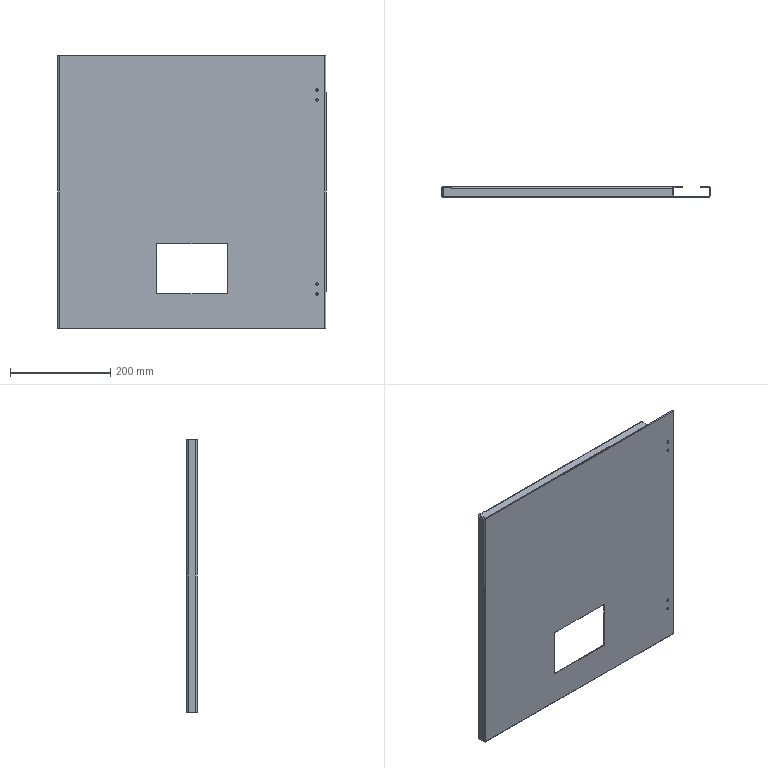Part | NX | features BREP 1 | 1 solid | 78 faces | box 534.5 x 20 x 546 mm | volume 515019 mm3 | plane 56 | cylinder 22 | commonest cylinder face diameters 3 x8 5 x8 6 x6